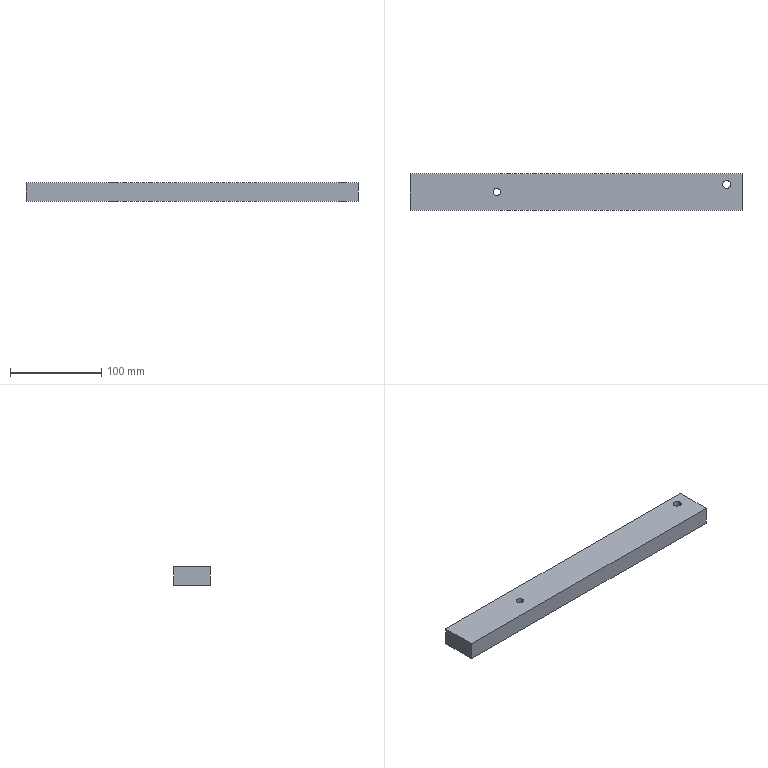Part | SolidWorks | features Cut 1, Extrusion 1, HoleWzd 1, ICE 1 | 1 solid | 10 faces | box 363 x 40 x 20 mm | volume 288260 mm3 | plane 6 | cylinder 4 | commonest cylinder face diameters 8 x2 8.5 x2
STEP:
#1=CARTESIAN_POINT('',(427.026,8.288,0.));
#2=VERTEX_POINT('',#1);
#3=CARTESIAN_POINT('',(435.526,8.288,0.));
#4=VERTEX_POINT('',#3);
#5=CARTESIAN_POINT('',(431.276,8.288,0.));
#6=DIRECTION('',(0.,0.,1.));
#7=DIRECTION('',(1.,0.,0.));
#8=AXIS2_PLACEMENT_3D('',#5,#6,#7);
#9=CIRCLE('',#8,4.25);
#10=EDGE_CURVE('',#2,#4,#9,.T.);
#11=ORIENTED_EDGE('',*,*,#10,.F.);
#12=CARTESIAN_POINT('',(427.026,8.288,20.));
#13=VERTEX_POINT('',#12);
#14=CARTESIAN_POINT('',(427.026,8.288,20.));
#15=DIRECTION('',(0.,0.,1.));
#16=VECTOR('',#15,1000.);
#17=LINE('',#14,#16);
#18=EDGE_CURVE('',#2,#13,#17,.T.);
#19=ORIENTED_EDGE('',*,*,#18,.T.);
#20=CARTESIAN_POINT('',(435.526,8.288,20.));
#21=VERTEX_POINT('',#20);
#22=CARTESIAN_POINT('',(431.276,8.288,20.));
#23=DIRECTION('',(0.,0.,1.));
#24=DIRECTION('',(1.,0.,0.));
#25=AXIS2_PLACEMENT_3D('',#22,#23,#24);
#26=CIRCLE('',#25,4.25);
#27=EDGE_CURVE('',#13,#21,#26,.T.);
#28=ORIENTED_EDGE('',*,*,#27,.T.);
#29=CARTESIAN_POINT('',(435.526,8.288,20.));
#30=DIRECTION('',(0.,0.,1.));
#31=VECTOR('',#30,1000.);
#32=LINE('',#29,#31);
#33=EDGE_CURVE('',#4,#21,#32,.T.);
#34=ORIENTED_EDGE('',*,*,#33,.F.);
#35=EDGE_LOOP('',(#11,#19,#28,#34));
#36=FACE_OUTER_BOUND('',#35,.T.);
#37=CARTESIAN_POINT('',(431.276,8.288,20.));
#38=DIRECTION('',(0.,0.,1.));
#39=DIRECTION('',(1.,0.,0.));
#40=AXIS2_PLACEMENT_3D('',#37,#38,#39);
#41=CYLINDRICAL_SURFACE('',#40,4.25);
#42=ADVANCED_FACE('',(#36),#41,.F.);
#43=CARTESIAN_POINT('',(176.,0.,20.));
#44=VERTEX_POINT('',#43);
#45=CARTESIAN_POINT('',(184.,0.,20.));
#46=VERTEX_POINT('',#45);
#47=CARTESIAN_POINT('',(180.,0.,20.));
#48=DIRECTION('',(0.,0.,1.));
#49=DIRECTION('',(1.,0.,0.));
#50=AXIS2_PLACEMENT_3D('',#47,#48,#49);
#51=CIRCLE('',#50,4.);
#52=EDGE_CURVE('',#44,#46,#51,.T.);
#53=ORIENTED_EDGE('',*,*,#52,.T.);
#54=CARTESIAN_POINT('',(184.,0.,0.));
#55=VERTEX_POINT('',#54);
#56=CARTESIAN_POINT('',(184.,0.,20.));
#57=DIRECTION('',(0.,0.,-1.));
#58=VECTOR('',#57,1000.);
#59=LINE('',#56,#58);
#60=EDGE_CURVE('',#46,#55,#59,.T.);
#61=ORIENTED_EDGE('',*,*,#60,.T.);
#62=CARTESIAN_POINT('',(176.,0.,0.));
#63=VERTEX_POINT('',#62);
#64=CARTESIAN_POINT('',(180.,0.,0.));
#65=DIRECTION('',(0.,0.,1.));
#66=DIRECTION('',(1.,0.,0.));
#67=AXIS2_PLACEMENT_3D('',#64,#65,#66);
#68=CIRCLE('',#67,4.);
#69=EDGE_CURVE('',#63,#55,#68,.T.);
#70=ORIENTED_EDGE('',*,*,#69,.F.);
#71=CARTESIAN_POINT('',(176.,0.,20.));
#72=DIRECTION('',(0.,0.,-1.));
#73=VECTOR('',#72,1000.);
#74=LINE('',#71,#73);
#75=EDGE_CURVE('',#44,#63,#74,.T.);
#76=ORIENTED_EDGE('',*,*,#75,.F.);
#77=EDGE_LOOP('',(#53,#61,#70,#76));
#78=FACE_OUTER_BOUND('',#77,.T.);
#79=CARTESIAN_POINT('',(180.,0.,20.));
#80=DIRECTION('',(0.,0.,-1.));
#81=DIRECTION('',(-1.,0.,0.));
#82=AXIS2_PLACEMENT_3D('',#79,#80,#81);
#83=CYLINDRICAL_SURFACE('',#82,4.);
#84=ADVANCED_FACE('',(#78),#83,.F.);
#85=CARTESIAN_POINT('',(431.276,8.288,20.));
#86=DIRECTION('',(0.,0.,1.));
#87=DIRECTION('',(1.,0.,0.));
#88=AXIS2_PLACEMENT_3D('',#85,#86,#87);
#89=CIRCLE('',#88,4.25);
#90=EDGE_CURVE('',#21,#13,#89,.T.);
#91=ORIENTED_EDGE('',*,*,#90,.F.);
#92=ORIENTED_EDGE('',*,*,#27,.F.);
#93=EDGE_LOOP('',(#91,#92));
#94=FACE_BOUND('',#93,.T.);
#95=ORIENTED_EDGE('',*,*,#52,.F.);
#96=CARTESIAN_POINT('',(180.,0.,20.));
#97=DIRECTION('',(0.,0.,1.));
#98=DIRECTION('',(1.,0.,0.));
#99=AXIS2_PLACEMENT_3D('',#96,#97,#98);
#100=CIRCLE('',#99,4.);
#101=EDGE_CURVE('',#46,#44,#100,.T.);
#102=ORIENTED_EDGE('',*,*,#101,.F.);
#103=EDGE_LOOP('',(#95,#102));
#104=FACE_BOUND('',#103,.T.);
#105=CARTESIAN_POINT('',(448.,20.,20.));
#106=VERTEX_POINT('',#105);
#107=CARTESIAN_POINT('',(85.,20.,20.));
#108=VERTEX_POINT('',#107);
#109=CARTESIAN_POINT('',(-200.,20.,20.));
#110=DIRECTION('',(-1.,0.,0.));
#111=VECTOR('',#110,1000.);
#112=LINE('',#109,#111);
#113=EDGE_CURVE('',#106,#108,#112,.T.);
#114=ORIENTED_EDGE('',*,*,#113,.T.);
#115=CARTESIAN_POINT('',(85.,-20.,20.));
#116=VERTEX_POINT('',#115);
#117=CARTESIAN_POINT('',(85.,-20.,20.));
#118=DIRECTION('',(0.,1.,0.));
#119=VECTOR('',#118,1000.);
#120=LINE('',#117,#119);
#121=EDGE_CURVE('',#116,#108,#120,.T.);
#122=ORIENTED_EDGE('',*,*,#121,.F.);
#123=CARTESIAN_POINT('',(448.,-20.,20.));
#124=VERTEX_POINT('',#123);
#125=CARTESIAN_POINT('',(-200.,-20.,20.));
#126=DIRECTION('',(1.,0.,0.));
#127=VECTOR('',#126,1000.);
#128=LINE('',#125,#127);
#129=EDGE_CURVE('',#116,#124,#128,.T.);
#130=ORIENTED_EDGE('',*,*,#129,.T.);
#131=CARTESIAN_POINT('',(448.,20.,20.));
#132=DIRECTION('',(0.,-1.,0.));
#133=VECTOR('',#132,1000.);
#134=LINE('',#131,#133);
#135=EDGE_CURVE('',#106,#124,#134,.T.);
#136=ORIENTED_EDGE('',*,*,#135,.F.);
#137=EDGE_LOOP('',(#114,#122,#130,#136));
#138=FACE_OUTER_BOUND('',#137,.T.);
#139=CARTESIAN_POINT('',(0.,0.,20.));
#140=DIRECTION('',(0.,0.,1.));
#141=DIRECTION('',(1.,0.,0.));
#142=AXIS2_PLACEMENT_3D('',#139,#140,#141);
#143=PLANE('',#142);
#144=ADVANCED_FACE('',(#94,#104,#138),#143,.T.);
#145=ORIENTED_EDGE('',*,*,#69,.T.);
#146=CARTESIAN_POINT('',(180.,0.,0.));
#147=DIRECTION('',(0.,0.,1.));
#148=DIRECTION('',(1.,0.,0.));
#149=AXIS2_PLACEMENT_3D('',#146,#147,#148);
#150=CIRCLE('',#149,4.);
#151=EDGE_CURVE('',#55,#63,#150,.T.);
#152=ORIENTED_EDGE('',*,*,#151,.T.);
#153=EDGE_LOOP('',(#145,#152));
#154=FACE_BOUND('',#153,.T.);
#155=CARTESIAN_POINT('',(431.276,8.288,0.));
#156=DIRECTION('',(0.,0.,1.));
#157=DIRECTION('',(1.,0.,0.));
#158=AXIS2_PLACEMENT_3D('',#155,#156,#157);
#159=CIRCLE('',#158,4.25);
#160=EDGE_CURVE('',#4,#2,#159,.T.);
#161=ORIENTED_EDGE('',*,*,#160,.T.);
#162=ORIENTED_EDGE('',*,*,#10,.T.);
#163=EDGE_LOOP('',(#161,#162));
#164=FACE_BOUND('',#163,.T.);
#165=CARTESIAN_POINT('',(85.,20.,0.));
#166=VERTEX_POINT('',#165);
#167=CARTESIAN_POINT('',(85.,-20.,0.));
#168=VERTEX_POINT('',#167);
#169=CARTESIAN_POINT('',(85.,20.,0.));
#170=DIRECTION('',(0.,-1.,0.));
#171=VECTOR('',#170,1000.);
#172=LINE('',#169,#171);
#173=EDGE_CURVE('',#166,#168,#172,.T.);
#174=ORIENTED_EDGE('',*,*,#173,.F.);
#175=CARTESIAN_POINT('',(448.,20.,0.));
#176=VERTEX_POINT('',#175);
#177=CARTESIAN_POINT('',(-200.,20.,0.));
#178=DIRECTION('',(-1.,0.,0.));
#179=VECTOR('',#178,1000.);
#180=LINE('',#177,#179);
#181=EDGE_CURVE('',#176,#166,#180,.T.);
#182=ORIENTED_EDGE('',*,*,#181,.F.);
#183=CARTESIAN_POINT('',(448.,-20.,0.));
#184=VERTEX_POINT('',#183);
#185=CARTESIAN_POINT('',(448.,-20.,0.));
#186=DIRECTION('',(0.,1.,0.));
#187=VECTOR('',#186,1000.);
#188=LINE('',#185,#187);
#189=EDGE_CURVE('',#184,#176,#188,.T.);
#190=ORIENTED_EDGE('',*,*,#189,.F.);
#191=CARTESIAN_POINT('',(-200.,-20.,0.));
#192=DIRECTION('',(1.,0.,0.));
#193=VECTOR('',#192,1000.);
#194=LINE('',#191,#193);
#195=EDGE_CURVE('',#168,#184,#194,.T.);
#196=ORIENTED_EDGE('',*,*,#195,.F.);
#197=EDGE_LOOP('',(#174,#182,#190,#196));
#198=FACE_OUTER_BOUND('',#197,.T.);
#199=CARTESIAN_POINT('',(0.,0.,0.));
#200=DIRECTION('',(0.,0.,1.));
#201=DIRECTION('',(1.,0.,0.));
#202=AXIS2_PLACEMENT_3D('',#199,#200,#201);
#203=PLANE('',#202);
#204=ADVANCED_FACE('',(#154,#164,#198),#203,.F.);
#205=CARTESIAN_POINT('',(85.,20.,20.));
#206=DIRECTION('',(0.,0.,-1.));
#207=VECTOR('',#206,1000.);
#208=LINE('',#205,#207);
#209=EDGE_CURVE('',#108,#166,#208,.T.);
#210=ORIENTED_EDGE('',*,*,#209,.F.);
#211=ORIENTED_EDGE('',*,*,#113,.F.);
#212=CARTESIAN_POINT('',(448.,20.,0.));
#213=DIRECTION('',(0.,0.,1.));
#214=VECTOR('',#213,1000.);
#215=LINE('',#212,#214);
#216=EDGE_CURVE('',#176,#106,#215,.T.);
#217=ORIENTED_EDGE('',*,*,#216,.F.);
#218=ORIENTED_EDGE('',*,*,#181,.T.);
#219=EDGE_LOOP('',(#210,#211,#217,#218));
#220=FACE_OUTER_BOUND('',#219,.T.);
#221=CARTESIAN_POINT('',(-200.,20.,20.));
#222=DIRECTION('',(0.,-1.,0.));
#223=DIRECTION('',(0.,0.,-1.));
#224=AXIS2_PLACEMENT_3D('',#221,#222,#223);
#225=PLANE('',#224);
#226=ADVANCED_FACE('',(#220),#225,.F.);
#227=CARTESIAN_POINT('',(85.,-20.,0.));
#228=DIRECTION('',(0.,0.,1.));
#229=VECTOR('',#228,1000.);
#230=LINE('',#227,#229);
#231=EDGE_CURVE('',#168,#116,#230,.T.);
#232=ORIENTED_EDGE('',*,*,#231,.F.);
#233=ORIENTED_EDGE('',*,*,#195,.T.);
#234=CARTESIAN_POINT('',(448.,-20.,20.));
#235=DIRECTION('',(0.,0.,-1.));
#236=VECTOR('',#235,1000.);
#237=LINE('',#234,#236);
#238=EDGE_CURVE('',#124,#184,#237,.T.);
#239=ORIENTED_EDGE('',*,*,#238,.F.);
#240=ORIENTED_EDGE('',*,*,#129,.F.);
#241=EDGE_LOOP('',(#232,#233,#239,#240));
#242=FACE_OUTER_BOUND('',#241,.T.);
#243=CARTESIAN_POINT('',(-200.,-20.,20.));
#244=DIRECTION('',(0.,1.,0.));
#245=DIRECTION('',(0.,0.,1.));
#246=AXIS2_PLACEMENT_3D('',#243,#244,#245);
#247=PLANE('',#246);
#248=ADVANCED_FACE('',(#242),#247,.F.);
#249=ORIENTED_EDGE('',*,*,#60,.F.);
#250=ORIENTED_EDGE('',*,*,#101,.T.);
#251=ORIENTED_EDGE('',*,*,#75,.T.);
#252=ORIENTED_EDGE('',*,*,#151,.F.);
#253=EDGE_LOOP('',(#249,#250,#251,#252));
#254=FACE_OUTER_BOUND('',#253,.T.);
#255=CARTESIAN_POINT('',(180.,0.,20.));
#256=DIRECTION('',(0.,0.,-1.));
#257=DIRECTION('',(-1.,0.,0.));
#258=AXIS2_PLACEMENT_3D('',#255,#256,#257);
#259=CYLINDRICAL_SURFACE('',#258,4.);
#260=ADVANCED_FACE('',(#254),#259,.F.);
#261=ORIENTED_EDGE('',*,*,#238,.T.);
#262=ORIENTED_EDGE('',*,*,#189,.T.);
#263=ORIENTED_EDGE('',*,*,#216,.T.);
#264=ORIENTED_EDGE('',*,*,#135,.T.);
#265=EDGE_LOOP('',(#261,#262,#263,#264));
#266=FACE_OUTER_BOUND('',#265,.T.);
#267=CARTESIAN_POINT('',(448.,0.,0.));
#268=DIRECTION('',(1.,0.,0.));
#269=DIRECTION('',(0.,0.,-1.));
#270=AXIS2_PLACEMENT_3D('',#267,#268,#269);
#271=PLANE('',#270);
#272=ADVANCED_FACE('',(#266),#271,.T.);
#273=ORIENTED_EDGE('',*,*,#18,.F.);
#274=ORIENTED_EDGE('',*,*,#160,.F.);
#275=ORIENTED_EDGE('',*,*,#33,.T.);
#276=ORIENTED_EDGE('',*,*,#90,.T.);
#277=EDGE_LOOP('',(#273,#274,#275,#276));
#278=FACE_OUTER_BOUND('',#277,.T.);
#279=CARTESIAN_POINT('',(431.276,8.288,20.));
#280=DIRECTION('',(0.,0.,1.));
#281=DIRECTION('',(1.,0.,0.));
#282=AXIS2_PLACEMENT_3D('',#279,#280,#281);
#283=CYLINDRICAL_SURFACE('',#282,4.25);
#284=ADVANCED_FACE('',(#278),#283,.F.);
#285=ORIENTED_EDGE('',*,*,#209,.T.);
#286=ORIENTED_EDGE('',*,*,#173,.T.);
#287=ORIENTED_EDGE('',*,*,#231,.T.);
#288=ORIENTED_EDGE('',*,*,#121,.T.);
#289=EDGE_LOOP('',(#285,#286,#287,#288));
#290=FACE_OUTER_BOUND('',#289,.T.);
#291=CARTESIAN_POINT('',(85.,0.,0.));
#292=DIRECTION('',(-1.,0.,0.));
#293=DIRECTION('',(0.,0.,1.));
#294=AXIS2_PLACEMENT_3D('',#291,#292,#293);
#295=PLANE('',#294);
#296=ADVANCED_FACE('',(#290),#295,.T.);
#297=CLOSED_SHELL('',(#42,#84,#144,#204,#226,#248,#260,#272,#284,#296));
#298=MANIFOLD_SOLID_BREP('',#297);
#299=CARTESIAN_POINT('',(0.,0.,0.));
#300=DIRECTION('',(0.,0.,1.));
#301=DIRECTION('',(1.,0.,0.));
#302=AXIS2_PLACEMENT_3D('',#299,#300,#301);
#303=(LENGTH_UNIT()NAMED_UNIT(*)SI_UNIT(.MILLI.,.METRE.));
#304=UNCERTAINTY_MEASURE_WITH_UNIT(LENGTH_MEASURE(0.00001),#303,'','');
#305=(NAMED_UNIT(*)PLANE_ANGLE_UNIT()SI_UNIT($,.RADIAN.));
#306=(NAMED_UNIT(*)SI_UNIT($,.STERADIAN.)SOLID_ANGLE_UNIT());
#307=(GEOMETRIC_REPRESENTATION_CONTEXT(3)GLOBAL_UNCERTAINTY_ASSIGNED_CONTEXT((#304))GLOBAL_UNIT_ASSIGNED_CONTEXT((#303,#305,#306))REPRESENTATION_CONTEXT('',''));
#308=ADVANCED_BREP_SHAPE_REPRESENTATION('',(#298,#302),#307);